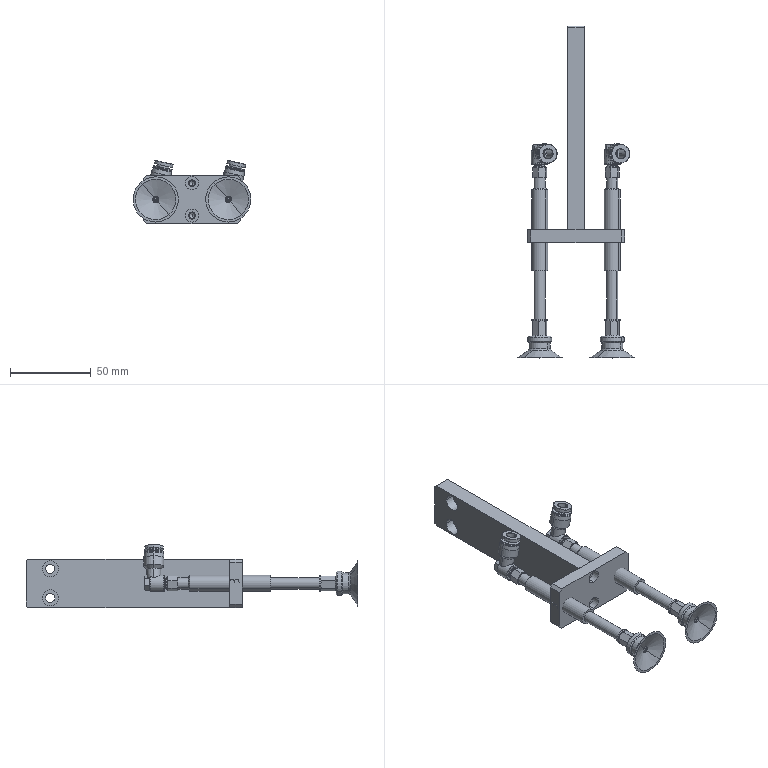Part | 10 solids | 534 faces | box 73 x 205.5 x 39.172 mm | volume 70978 mm3 | cone 198 | plane 160 | cylinder 146 | spline 30 | commonest cylinder face diameters 5 x12 6 x12 7 x12 10 x12 4 x8 5.5 x8